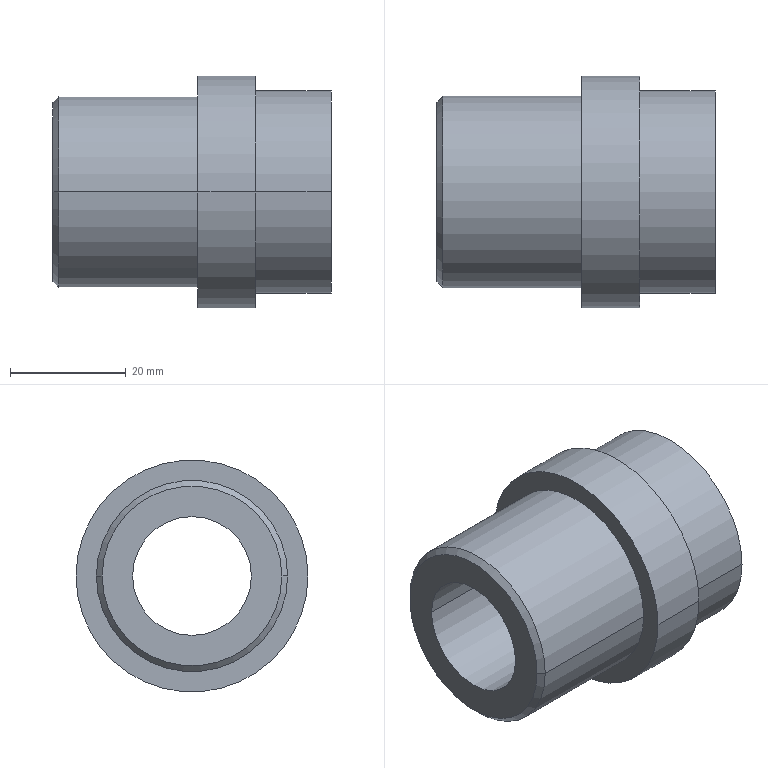Part | SolidWorks | features ICE 2, Revolution 1 | 1 solid | 17 faces | box 48 x 40 x 40 mm | volume 27829 mm3 | cylinder 10 | plane 5 | cone 2 | commonest cylinder face diameters 20.5 x2 24.378 x2 33 x2 35 x2 40 x2
STEP:
#1=CARTESIAN_POINT('',(-20.,-12.189,0.));
#2=VERTEX_POINT('',#1);
#3=CARTESIAN_POINT('',(-20.,12.189,0.));
#4=VERTEX_POINT('',#3);
#5=CARTESIAN_POINT('',(-20.,0.,0.));
#6=DIRECTION('',(1.,0.,0.));
#7=DIRECTION('',(0.,1.,0.));
#8=AXIS2_PLACEMENT_3D('',#5,#6,#7);
#9=CIRCLE('',#8,12.189);
#10=EDGE_CURVE('',#2,#4,#9,.T.);
#11=ORIENTED_EDGE('',*,*,#10,.F.);
#12=CARTESIAN_POINT('',(0.,-12.189,0.));
#13=VERTEX_POINT('',#12);
#14=CARTESIAN_POINT('',(-20.,-12.189,0.));
#15=DIRECTION('',(1.,0.,0.));
#16=VECTOR('',#15,1000.);
#17=LINE('',#14,#16);
#18=EDGE_CURVE('',#2,#13,#17,.T.);
#19=ORIENTED_EDGE('',*,*,#18,.T.);
#20=CARTESIAN_POINT('',(0.,12.189,0.));
#21=VERTEX_POINT('',#20);
#22=CARTESIAN_POINT('',(0.,0.,0.));
#23=DIRECTION('',(1.,0.,0.));
#24=DIRECTION('',(0.,1.,0.));
#25=AXIS2_PLACEMENT_3D('',#22,#23,#24);
#26=CIRCLE('',#25,12.189);
#27=EDGE_CURVE('',#13,#21,#26,.T.);
#28=ORIENTED_EDGE('',*,*,#27,.T.);
#29=CARTESIAN_POINT('',(-20.,12.189,0.));
#30=DIRECTION('',(1.,0.,0.));
#31=VECTOR('',#30,1000.);
#32=LINE('',#29,#31);
#33=EDGE_CURVE('',#4,#21,#32,.T.);
#34=ORIENTED_EDGE('',*,*,#33,.F.);
#35=EDGE_LOOP('',(#11,#19,#28,#34));
#36=FACE_OUTER_BOUND('',#35,.T.);
#37=CARTESIAN_POINT('',(-20.,0.,0.));
#38=DIRECTION('',(1.,0.,0.));
#39=DIRECTION('',(0.,1.,0.));
#40=AXIS2_PLACEMENT_3D('',#37,#38,#39);
#41=CYLINDRICAL_SURFACE('',#40,12.189);
#42=ADVANCED_FACE('',(#36),#41,.F.);
#43=CARTESIAN_POINT('',(-13.,17.5,0.));
#44=VERTEX_POINT('',#43);
#45=CARTESIAN_POINT('',(-13.,-17.5,0.));
#46=VERTEX_POINT('',#45);
#47=CARTESIAN_POINT('',(-13.,0.,0.));
#48=DIRECTION('',(1.,0.,0.));
#49=DIRECTION('',(0.,1.,0.));
#50=AXIS2_PLACEMENT_3D('',#47,#48,#49);
#51=CIRCLE('',#50,17.5);
#52=EDGE_CURVE('',#44,#46,#51,.T.);
#53=ORIENTED_EDGE('',*,*,#52,.T.);
#54=CARTESIAN_POINT('',(0.,-17.5,0.));
#55=VERTEX_POINT('',#54);
#56=CARTESIAN_POINT('',(0.,-17.5,0.));
#57=DIRECTION('',(1.,0.,0.));
#58=VECTOR('',#57,1000.);
#59=LINE('',#56,#58);
#60=EDGE_CURVE('',#46,#55,#59,.T.);
#61=ORIENTED_EDGE('',*,*,#60,.T.);
#62=CARTESIAN_POINT('',(0.,17.5,0.));
#63=VERTEX_POINT('',#62);
#64=CARTESIAN_POINT('',(0.,0.,0.));
#65=DIRECTION('',(1.,0.,0.));
#66=DIRECTION('',(0.,1.,0.));
#67=AXIS2_PLACEMENT_3D('',#64,#65,#66);
#68=CIRCLE('',#67,17.5);
#69=EDGE_CURVE('',#63,#55,#68,.T.);
#70=ORIENTED_EDGE('',*,*,#69,.F.);
#71=CARTESIAN_POINT('',(0.,17.5,0.));
#72=DIRECTION('',(1.,0.,0.));
#73=VECTOR('',#72,1000.);
#74=LINE('',#71,#73);
#75=EDGE_CURVE('',#44,#63,#74,.T.);
#76=ORIENTED_EDGE('',*,*,#75,.F.);
#77=EDGE_LOOP('',(#53,#61,#70,#76));
#78=FACE_OUTER_BOUND('',#77,.T.);
#79=CARTESIAN_POINT('',(0.,0.,0.));
#80=DIRECTION('',(1.,0.,0.));
#81=DIRECTION('',(0.,1.,0.));
#82=AXIS2_PLACEMENT_3D('',#79,#80,#81);
#83=CYLINDRICAL_SURFACE('',#82,17.5);
#84=ADVANCED_FACE('',(#78),#83,.T.);
#85=CARTESIAN_POINT('',(-23.,20.,0.));
#86=VERTEX_POINT('',#85);
#87=CARTESIAN_POINT('',(-23.,-20.,0.));
#88=VERTEX_POINT('',#87);
#89=CARTESIAN_POINT('',(-23.,0.,0.));
#90=DIRECTION('',(1.,0.,0.));
#91=DIRECTION('',(0.,1.,0.));
#92=AXIS2_PLACEMENT_3D('',#89,#90,#91);
#93=CIRCLE('',#92,20.);
#94=EDGE_CURVE('',#86,#88,#93,.T.);
#95=ORIENTED_EDGE('',*,*,#94,.T.);
#96=CARTESIAN_POINT('',(-13.,-20.,0.));
#97=VERTEX_POINT('',#96);
#98=CARTESIAN_POINT('',(0.,-20.,0.));
#99=DIRECTION('',(1.,0.,0.));
#100=VECTOR('',#99,1000.);
#101=LINE('',#98,#100);
#102=EDGE_CURVE('',#88,#97,#101,.T.);
#103=ORIENTED_EDGE('',*,*,#102,.T.);
#104=CARTESIAN_POINT('',(-13.,20.,0.));
#105=VERTEX_POINT('',#104);
#106=CARTESIAN_POINT('',(-13.,0.,0.));
#107=DIRECTION('',(1.,0.,0.));
#108=DIRECTION('',(0.,1.,0.));
#109=AXIS2_PLACEMENT_3D('',#106,#107,#108);
#110=CIRCLE('',#109,20.);
#111=EDGE_CURVE('',#105,#97,#110,.T.);
#112=ORIENTED_EDGE('',*,*,#111,.F.);
#113=CARTESIAN_POINT('',(0.,20.,0.));
#114=DIRECTION('',(1.,0.,0.));
#115=VECTOR('',#114,1000.);
#116=LINE('',#113,#115);
#117=EDGE_CURVE('',#86,#105,#116,.T.);
#118=ORIENTED_EDGE('',*,*,#117,.F.);
#119=EDGE_LOOP('',(#95,#103,#112,#118));
#120=FACE_OUTER_BOUND('',#119,.T.);
#121=CARTESIAN_POINT('',(0.,0.,0.));
#122=DIRECTION('',(1.,0.,0.));
#123=DIRECTION('',(0.,1.,0.));
#124=AXIS2_PLACEMENT_3D('',#121,#122,#123);
#125=CYLINDRICAL_SURFACE('',#124,20.);
#126=ADVANCED_FACE('',(#120),#125,.T.);
#127=CARTESIAN_POINT('',(-47.,16.5,0.));
#128=VERTEX_POINT('',#127);
#129=CARTESIAN_POINT('',(-47.,-16.5,0.));
#130=VERTEX_POINT('',#129);
#131=CARTESIAN_POINT('',(-47.,0.,0.));
#132=DIRECTION('',(1.,0.,0.));
#133=DIRECTION('',(0.,1.,0.));
#134=AXIS2_PLACEMENT_3D('',#131,#132,#133);
#135=CIRCLE('',#134,16.5);
#136=EDGE_CURVE('',#128,#130,#135,.T.);
#137=ORIENTED_EDGE('',*,*,#136,.T.);
#138=CARTESIAN_POINT('',(-23.,-16.5,0.));
#139=VERTEX_POINT('',#138);
#140=CARTESIAN_POINT('',(0.,-16.5,0.));
#141=DIRECTION('',(1.,0.,0.));
#142=VECTOR('',#141,1000.);
#143=LINE('',#140,#142);
#144=EDGE_CURVE('',#130,#139,#143,.T.);
#145=ORIENTED_EDGE('',*,*,#144,.T.);
#146=CARTESIAN_POINT('',(-23.,16.5,0.));
#147=VERTEX_POINT('',#146);
#148=CARTESIAN_POINT('',(-23.,0.,0.));
#149=DIRECTION('',(1.,0.,0.));
#150=DIRECTION('',(0.,1.,0.));
#151=AXIS2_PLACEMENT_3D('',#148,#149,#150);
#152=CIRCLE('',#151,16.5);
#153=EDGE_CURVE('',#147,#139,#152,.T.);
#154=ORIENTED_EDGE('',*,*,#153,.F.);
#155=CARTESIAN_POINT('',(0.,16.5,0.));
#156=DIRECTION('',(1.,0.,0.));
#157=VECTOR('',#156,1000.);
#158=LINE('',#155,#157);
#159=EDGE_CURVE('',#128,#147,#158,.T.);
#160=ORIENTED_EDGE('',*,*,#159,.F.);
#161=EDGE_LOOP('',(#137,#145,#154,#160));
#162=FACE_OUTER_BOUND('',#161,.T.);
#163=CARTESIAN_POINT('',(0.,0.,0.));
#164=DIRECTION('',(1.,0.,0.));
#165=DIRECTION('',(0.,1.,0.));
#166=AXIS2_PLACEMENT_3D('',#163,#164,#165);
#167=CYLINDRICAL_SURFACE('',#166,16.5);
#168=ADVANCED_FACE('',(#162),#167,.T.);
#169=CARTESIAN_POINT('',(-48.,15.5,0.));
#170=VERTEX_POINT('',#169);
#171=CARTESIAN_POINT('',(-48.,-15.5,0.));
#172=VERTEX_POINT('',#171);
#173=CARTESIAN_POINT('',(-48.,0.,0.));
#174=DIRECTION('',(1.,0.,0.));
#175=DIRECTION('',(0.,1.,0.));
#176=AXIS2_PLACEMENT_3D('',#173,#174,#175);
#177=CIRCLE('',#176,15.5);
#178=EDGE_CURVE('',#170,#172,#177,.T.);
#179=ORIENTED_EDGE('',*,*,#178,.T.);
#180=CARTESIAN_POINT('',(-47.,-16.5,0.));
#181=DIRECTION('',(0.7071,-0.7071,0.));
#182=VECTOR('',#181,1000.);
#183=LINE('',#180,#182);
#184=EDGE_CURVE('',#172,#130,#183,.T.);
#185=ORIENTED_EDGE('',*,*,#184,.T.);
#186=ORIENTED_EDGE('',*,*,#136,.F.);
#187=CARTESIAN_POINT('',(-47.,16.5,0.));
#188=DIRECTION('',(0.7071,0.7071,0.));
#189=VECTOR('',#188,1000.);
#190=LINE('',#187,#189);
#191=EDGE_CURVE('',#170,#128,#190,.T.);
#192=ORIENTED_EDGE('',*,*,#191,.F.);
#193=EDGE_LOOP('',(#179,#185,#186,#192));
#194=FACE_OUTER_BOUND('',#193,.T.);
#195=CARTESIAN_POINT('',(-47.,0.,0.));
#196=DIRECTION('',(1.,0.,0.));
#197=DIRECTION('',(0.,1.,0.));
#198=AXIS2_PLACEMENT_3D('',#195,#196,#197);
#199=CONICAL_SURFACE('',#198,16.5,0.7854);
#200=ADVANCED_FACE('',(#194),#199,.T.);
#201=CARTESIAN_POINT('',(-48.,-10.25,0.));
#202=VERTEX_POINT('',#201);
#203=CARTESIAN_POINT('',(-48.,10.25,0.));
#204=VERTEX_POINT('',#203);
#205=CARTESIAN_POINT('',(-48.,0.,0.));
#206=DIRECTION('',(1.,0.,0.));
#207=DIRECTION('',(0.,1.,0.));
#208=AXIS2_PLACEMENT_3D('',#205,#206,#207);
#209=CIRCLE('',#208,10.25);
#210=EDGE_CURVE('',#202,#204,#209,.T.);
#211=ORIENTED_EDGE('',*,*,#210,.F.);
#212=CARTESIAN_POINT('',(-20.,-10.25,0.));
#213=VERTEX_POINT('',#212);
#214=CARTESIAN_POINT('',(-48.,-10.25,0.));
#215=DIRECTION('',(1.,0.,0.));
#216=VECTOR('',#215,1000.);
#217=LINE('',#214,#216);
#218=EDGE_CURVE('',#202,#213,#217,.T.);
#219=ORIENTED_EDGE('',*,*,#218,.T.);
#220=CARTESIAN_POINT('',(-20.,10.25,0.));
#221=VERTEX_POINT('',#220);
#222=CARTESIAN_POINT('',(-20.,0.,0.));
#223=DIRECTION('',(-1.,0.,0.));
#224=DIRECTION('',(0.,1.,0.));
#225=AXIS2_PLACEMENT_3D('',#222,#223,#224);
#226=CIRCLE('',#225,10.25);
#227=EDGE_CURVE('',#221,#213,#226,.T.);
#228=ORIENTED_EDGE('',*,*,#227,.F.);
#229=CARTESIAN_POINT('',(-48.,10.25,0.));
#230=DIRECTION('',(1.,0.,0.));
#231=VECTOR('',#230,1000.);
#232=LINE('',#229,#231);
#233=EDGE_CURVE('',#204,#221,#232,.T.);
#234=ORIENTED_EDGE('',*,*,#233,.F.);
#235=EDGE_LOOP('',(#211,#219,#228,#234));
#236=FACE_OUTER_BOUND('',#235,.T.);
#237=CARTESIAN_POINT('',(-48.,0.,0.));
#238=DIRECTION('',(1.,0.,0.));
#239=DIRECTION('',(0.,1.,0.));
#240=AXIS2_PLACEMENT_3D('',#237,#238,#239);
#241=CYLINDRICAL_SURFACE('',#240,10.25);
#242=ADVANCED_FACE('',(#236),#241,.F.);
#243=ORIENTED_EDGE('',*,*,#218,.F.);
#244=CARTESIAN_POINT('',(-48.,0.,0.));
#245=DIRECTION('',(1.,0.,0.));
#246=DIRECTION('',(0.,1.,0.));
#247=AXIS2_PLACEMENT_3D('',#244,#245,#246);
#248=CIRCLE('',#247,10.25);
#249=EDGE_CURVE('',#204,#202,#248,.T.);
#250=ORIENTED_EDGE('',*,*,#249,.F.);
#251=ORIENTED_EDGE('',*,*,#233,.T.);
#252=CARTESIAN_POINT('',(-20.,0.,0.));
#253=DIRECTION('',(-1.,0.,0.));
#254=DIRECTION('',(0.,1.,0.));
#255=AXIS2_PLACEMENT_3D('',#252,#253,#254);
#256=CIRCLE('',#255,10.25);
#257=EDGE_CURVE('',#213,#221,#256,.T.);
#258=ORIENTED_EDGE('',*,*,#257,.F.);
#259=EDGE_LOOP('',(#243,#250,#251,#258));
#260=FACE_OUTER_BOUND('',#259,.T.);
#261=CARTESIAN_POINT('',(-48.,0.,0.));
#262=DIRECTION('',(1.,0.,0.));
#263=DIRECTION('',(0.,1.,0.));
#264=AXIS2_PLACEMENT_3D('',#261,#262,#263);
#265=CYLINDRICAL_SURFACE('',#264,10.25);
#266=ADVANCED_FACE('',(#260),#265,.F.);
#267=ORIENTED_EDGE('',*,*,#249,.T.);
#268=ORIENTED_EDGE('',*,*,#210,.T.);
#269=EDGE_LOOP('',(#267,#268));
#270=FACE_BOUND('',#269,.T.);
#271=ORIENTED_EDGE('',*,*,#178,.F.);
#272=CARTESIAN_POINT('',(-48.,0.,0.));
#273=DIRECTION('',(1.,0.,0.));
#274=DIRECTION('',(0.,1.,0.));
#275=AXIS2_PLACEMENT_3D('',#272,#273,#274);
#276=CIRCLE('',#275,15.5);
#277=EDGE_CURVE('',#172,#170,#276,.T.);
#278=ORIENTED_EDGE('',*,*,#277,.F.);
#279=EDGE_LOOP('',(#271,#278));
#280=FACE_OUTER_BOUND('',#279,.T.);
#281=CARTESIAN_POINT('',(-48.,0.,0.));
#282=DIRECTION('',(-1.,0.,0.));
#283=DIRECTION('',(0.,-1.,0.));
#284=AXIS2_PLACEMENT_3D('',#281,#282,#283);
#285=PLANE('',#284);
#286=ADVANCED_FACE('',(#270,#280),#285,.T.);
#287=ORIENTED_EDGE('',*,*,#184,.F.);
#288=ORIENTED_EDGE('',*,*,#277,.T.);
#289=ORIENTED_EDGE('',*,*,#191,.T.);
#290=CARTESIAN_POINT('',(-47.,0.,0.));
#291=DIRECTION('',(1.,0.,0.));
#292=DIRECTION('',(0.,1.,0.));
#293=AXIS2_PLACEMENT_3D('',#290,#291,#292);
#294=CIRCLE('',#293,16.5);
#295=EDGE_CURVE('',#130,#128,#294,.T.);
#296=ORIENTED_EDGE('',*,*,#295,.F.);
#297=EDGE_LOOP('',(#287,#288,#289,#296));
#298=FACE_OUTER_BOUND('',#297,.T.);
#299=CARTESIAN_POINT('',(-47.,0.,0.));
#300=DIRECTION('',(1.,0.,0.));
#301=DIRECTION('',(0.,1.,0.));
#302=AXIS2_PLACEMENT_3D('',#299,#300,#301);
#303=CONICAL_SURFACE('',#302,16.5,0.7854);
#304=ADVANCED_FACE('',(#298),#303,.T.);
#305=ORIENTED_EDGE('',*,*,#144,.F.);
#306=ORIENTED_EDGE('',*,*,#295,.T.);
#307=ORIENTED_EDGE('',*,*,#159,.T.);
#308=CARTESIAN_POINT('',(-23.,0.,0.));
#309=DIRECTION('',(1.,0.,0.));
#310=DIRECTION('',(0.,1.,0.));
#311=AXIS2_PLACEMENT_3D('',#308,#309,#310);
#312=CIRCLE('',#311,16.5);
#313=EDGE_CURVE('',#139,#147,#312,.T.);
#314=ORIENTED_EDGE('',*,*,#313,.F.);
#315=EDGE_LOOP('',(#305,#306,#307,#314));
#316=FACE_OUTER_BOUND('',#315,.T.);
#317=CARTESIAN_POINT('',(0.,0.,0.));
#318=DIRECTION('',(1.,0.,0.));
#319=DIRECTION('',(0.,1.,0.));
#320=AXIS2_PLACEMENT_3D('',#317,#318,#319);
#321=CYLINDRICAL_SURFACE('',#320,16.5);
#322=ADVANCED_FACE('',(#316),#321,.T.);
#323=ORIENTED_EDGE('',*,*,#153,.T.);
#324=ORIENTED_EDGE('',*,*,#313,.T.);
#325=EDGE_LOOP('',(#323,#324));
#326=FACE_BOUND('',#325,.T.);
#327=ORIENTED_EDGE('',*,*,#94,.F.);
#328=CARTESIAN_POINT('',(-23.,0.,0.));
#329=DIRECTION('',(1.,0.,0.));
#330=DIRECTION('',(0.,1.,0.));
#331=AXIS2_PLACEMENT_3D('',#328,#329,#330);
#332=CIRCLE('',#331,20.);
#333=EDGE_CURVE('',#88,#86,#332,.T.);
#334=ORIENTED_EDGE('',*,*,#333,.F.);
#335=EDGE_LOOP('',(#327,#334));
#336=FACE_OUTER_BOUND('',#335,.T.);
#337=CARTESIAN_POINT('',(-23.,16.5,0.));
#338=DIRECTION('',(-1.,0.,0.));
#339=DIRECTION('',(0.,-1.,0.));
#340=AXIS2_PLACEMENT_3D('',#337,#338,#339);
#341=PLANE('',#340);
#342=ADVANCED_FACE('',(#326,#336),#341,.T.);
#343=ORIENTED_EDGE('',*,*,#102,.F.);
#344=ORIENTED_EDGE('',*,*,#333,.T.);
#345=ORIENTED_EDGE('',*,*,#117,.T.);
#346=CARTESIAN_POINT('',(-13.,0.,0.));
#347=DIRECTION('',(1.,0.,0.));
#348=DIRECTION('',(0.,1.,0.));
#349=AXIS2_PLACEMENT_3D('',#346,#347,#348);
#350=CIRCLE('',#349,20.);
#351=EDGE_CURVE('',#97,#105,#350,.T.);
#352=ORIENTED_EDGE('',*,*,#351,.F.);
#353=EDGE_LOOP('',(#343,#344,#345,#352));
#354=FACE_OUTER_BOUND('',#353,.T.);
#355=CARTESIAN_POINT('',(0.,0.,0.));
#356=DIRECTION('',(1.,0.,0.));
#357=DIRECTION('',(0.,1.,0.));
#358=AXIS2_PLACEMENT_3D('',#355,#356,#357);
#359=CYLINDRICAL_SURFACE('',#358,20.);
#360=ADVANCED_FACE('',(#354),#359,.T.);
#361=ORIENTED_EDGE('',*,*,#111,.T.);
#362=ORIENTED_EDGE('',*,*,#351,.T.);
#363=EDGE_LOOP('',(#361,#362));
#364=FACE_OUTER_BOUND('',#363,.T.);
#365=ORIENTED_EDGE('',*,*,#52,.F.);
#366=CARTESIAN_POINT('',(-13.,0.,0.));
#367=DIRECTION('',(1.,0.,0.));
#368=DIRECTION('',(0.,1.,0.));
#369=AXIS2_PLACEMENT_3D('',#366,#367,#368);
#370=CIRCLE('',#369,17.5);
#371=EDGE_CURVE('',#46,#44,#370,.T.);
#372=ORIENTED_EDGE('',*,*,#371,.F.);
#373=EDGE_LOOP('',(#365,#372));
#374=FACE_BOUND('',#373,.T.);
#375=CARTESIAN_POINT('',(-13.,20.,0.));
#376=DIRECTION('',(1.,0.,0.));
#377=DIRECTION('',(0.,1.,0.));
#378=AXIS2_PLACEMENT_3D('',#375,#376,#377);
#379=PLANE('',#378);
#380=ADVANCED_FACE('',(#364,#374),#379,.T.);
#381=ORIENTED_EDGE('',*,*,#60,.F.);
#382=ORIENTED_EDGE('',*,*,#371,.T.);
#383=ORIENTED_EDGE('',*,*,#75,.T.);
#384=CARTESIAN_POINT('',(0.,0.,0.));
#385=DIRECTION('',(1.,0.,0.));
#386=DIRECTION('',(0.,1.,0.));
#387=AXIS2_PLACEMENT_3D('',#384,#385,#386);
#388=CIRCLE('',#387,17.5);
#389=EDGE_CURVE('',#55,#63,#388,.T.);
#390=ORIENTED_EDGE('',*,*,#389,.F.);
#391=EDGE_LOOP('',(#381,#382,#383,#390));
#392=FACE_OUTER_BOUND('',#391,.T.);
#393=CARTESIAN_POINT('',(0.,0.,0.));
#394=DIRECTION('',(1.,0.,0.));
#395=DIRECTION('',(0.,1.,0.));
#396=AXIS2_PLACEMENT_3D('',#393,#394,#395);
#397=CYLINDRICAL_SURFACE('',#396,17.5);
#398=ADVANCED_FACE('',(#392),#397,.T.);
#399=CARTESIAN_POINT('',(0.,0.,0.));
#400=DIRECTION('',(1.,0.,0.));
#401=DIRECTION('',(0.,1.,0.));
#402=AXIS2_PLACEMENT_3D('',#399,#400,#401);
#403=CIRCLE('',#402,12.189);
#404=EDGE_CURVE('',#21,#13,#403,.T.);
#405=ORIENTED_EDGE('',*,*,#404,.F.);
#406=ORIENTED_EDGE('',*,*,#27,.F.);
#407=EDGE_LOOP('',(#405,#406));
#408=FACE_BOUND('',#407,.T.);
#409=ORIENTED_EDGE('',*,*,#69,.T.);
#410=ORIENTED_EDGE('',*,*,#389,.T.);
#411=EDGE_LOOP('',(#409,#410));
#412=FACE_OUTER_BOUND('',#411,.T.);
#413=CARTESIAN_POINT('',(0.,17.5,0.));
#414=DIRECTION('',(1.,0.,0.));
#415=DIRECTION('',(0.,1.,0.));
#416=AXIS2_PLACEMENT_3D('',#413,#414,#415);
#417=PLANE('',#416);
#418=ADVANCED_FACE('',(#408,#412),#417,.T.);
#419=CARTESIAN_POINT('',(-20.,0.,0.));
#420=DIRECTION('',(1.,0.,0.));
#421=DIRECTION('',(0.,1.,0.));
#422=AXIS2_PLACEMENT_3D('',#419,#420,#421);
#423=CIRCLE('',#422,12.189);
#424=EDGE_CURVE('',#4,#2,#423,.T.);
#425=ORIENTED_EDGE('',*,*,#424,.T.);
#426=ORIENTED_EDGE('',*,*,#10,.T.);
#427=EDGE_LOOP('',(#425,#426));
#428=FACE_OUTER_BOUND('',#427,.T.);
#429=ORIENTED_EDGE('',*,*,#227,.T.);
#430=ORIENTED_EDGE('',*,*,#257,.T.);
#431=EDGE_LOOP('',(#429,#430));
#432=FACE_BOUND('',#431,.T.);
#433=CARTESIAN_POINT('',(-20.,0.,0.));
#434=DIRECTION('',(1.,0.,0.));
#435=DIRECTION('',(0.,1.,0.));
#436=AXIS2_PLACEMENT_3D('',#433,#434,#435);
#437=PLANE('',#436);
#438=ADVANCED_FACE('',(#428,#432),#437,.T.);
#439=ORIENTED_EDGE('',*,*,#18,.F.);
#440=ORIENTED_EDGE('',*,*,#424,.F.);
#441=ORIENTED_EDGE('',*,*,#33,.T.);
#442=ORIENTED_EDGE('',*,*,#404,.T.);
#443=EDGE_LOOP('',(#439,#440,#441,#442));
#444=FACE_OUTER_BOUND('',#443,.T.);
#445=CARTESIAN_POINT('',(-20.,0.,0.));
#446=DIRECTION('',(1.,0.,0.));
#447=DIRECTION('',(0.,1.,0.));
#448=AXIS2_PLACEMENT_3D('',#445,#446,#447);
#449=CYLINDRICAL_SURFACE('',#448,12.189);
#450=ADVANCED_FACE('',(#444),#449,.F.);
#451=CLOSED_SHELL('',(#42,#84,#126,#168,#200,#242,#266,#286,#304,#322,#342,#360,#380,#398,#418,#438,#450));
#452=MANIFOLD_SOLID_BREP('',#451);
#453=CARTESIAN_POINT('',(0.,0.,0.));
#454=DIRECTION('',(0.,0.,1.));
#455=DIRECTION('',(1.,0.,0.));
#456=AXIS2_PLACEMENT_3D('',#453,#454,#455);
#457=(LENGTH_UNIT()NAMED_UNIT(*)SI_UNIT(.MILLI.,.METRE.));
#458=UNCERTAINTY_MEASURE_WITH_UNIT(LENGTH_MEASURE(0.00001),#457,'','');
#459=(NAMED_UNIT(*)PLANE_ANGLE_UNIT()SI_UNIT($,.RADIAN.));
#460=(NAMED_UNIT(*)SI_UNIT($,.STERADIAN.)SOLID_ANGLE_UNIT());
#461=(GEOMETRIC_REPRESENTATION_CONTEXT(3)GLOBAL_UNCERTAINTY_ASSIGNED_CONTEXT((#458))GLOBAL_UNIT_ASSIGNED_CONTEXT((#457,#459,#460))REPRESENTATION_CONTEXT('',''));
#462=ADVANCED_BREP_SHAPE_REPRESENTATION('',(#452,#456),#461);